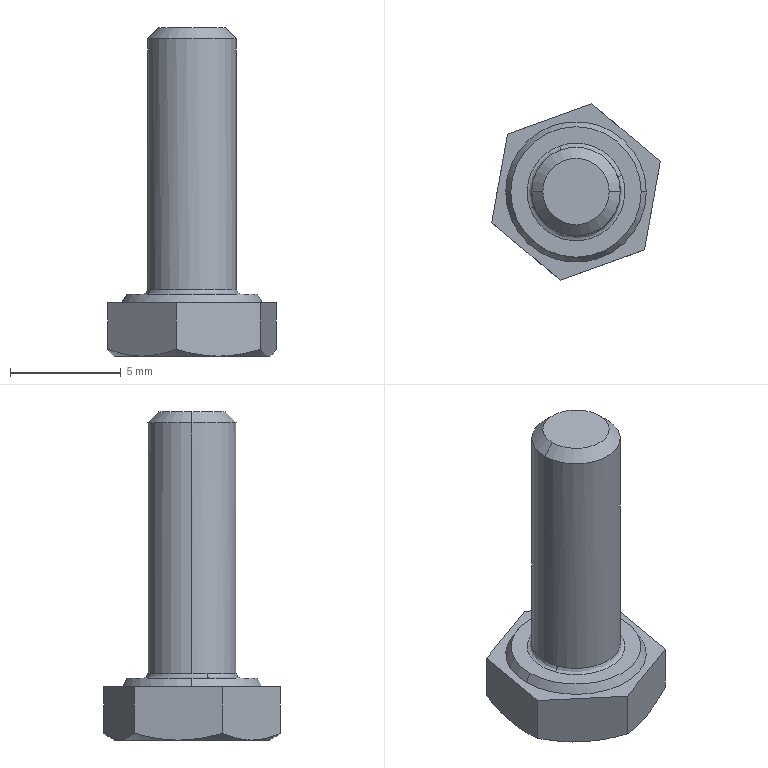Part | NX | features BREP 1 | 1 solid | 39 faces | box 7.602 x 7.957 x 14.8 mm | volume 249.931 mm3 | plane 23 | cone 11 | spline 3 | cylinder 2 | commonest cylinder face diameters 4 x2
STEP:
#1=CARTESIAN_POINT('',(-262.311,-178.403,2116.));
#2=VERTEX_POINT('',#1);
#3=CARTESIAN_POINT('',(-258.311,-178.403,2116.));
#4=VERTEX_POINT('',#3);
#5=CARTESIAN_POINT('',(-260.311,-178.403,2116.));
#6=DIRECTION('',(0.,0.,-1.));
#7=DIRECTION('',(-1.,0.,0.));
#8=AXIS2_PLACEMENT_3D('',#5,#6,#7);
#9=CIRCLE('',#8,2.);
#10=EDGE_CURVE('',#2,#4,#9,.T.);
#11=ORIENTED_EDGE('',*,*,#10,.T.);
#12=CARTESIAN_POINT('',(-258.311,-178.403,2104.7));
#13=VERTEX_POINT('',#12);
#14=CARTESIAN_POINT('',(-258.311,-178.403,2101.7));
#15=DIRECTION('',(0.,0.,-1.));
#16=VECTOR('',#15,1000.);
#17=LINE('',#14,#16);
#18=EDGE_CURVE('',#13,#4,#17,.F.);
#19=ORIENTED_EDGE('',*,*,#18,.F.);
#20=CARTESIAN_POINT('',(-258.429,-177.724,2104.7));
#21=VERTEX_POINT('',#20);
#22=CARTESIAN_POINT('',(-260.311,-178.403,2104.7));
#23=DIRECTION('',(0.,0.,1.));
#24=DIRECTION('',(-1.,0.,0.));
#25=AXIS2_PLACEMENT_3D('',#22,#23,#24);
#26=CIRCLE('',#25,2.);
#27=EDGE_CURVE('',#13,#21,#26,.T.);
#28=ORIENTED_EDGE('',*,*,#27,.T.);
#29=CARTESIAN_POINT('',(-260.99,-176.522,2104.7));
#30=VERTEX_POINT('',#29);
#31=CARTESIAN_POINT('',(-260.311,-178.403,2104.7));
#32=DIRECTION('',(0.,0.,1.));
#33=DIRECTION('',(-1.,0.,0.));
#34=AXIS2_PLACEMENT_3D('',#31,#32,#33);
#35=CIRCLE('',#34,2.);
#36=EDGE_CURVE('',#21,#30,#35,.T.);
#37=ORIENTED_EDGE('',*,*,#36,.T.);
#38=CARTESIAN_POINT('',(-262.311,-178.403,2104.7));
#39=VERTEX_POINT('',#38);
#40=CARTESIAN_POINT('',(-260.311,-178.403,2104.7));
#41=DIRECTION('',(0.,0.,1.));
#42=DIRECTION('',(-1.,0.,0.));
#43=AXIS2_PLACEMENT_3D('',#40,#41,#42);
#44=CIRCLE('',#43,2.);
#45=EDGE_CURVE('',#30,#39,#44,.T.);
#46=ORIENTED_EDGE('',*,*,#45,.T.);
#47=CARTESIAN_POINT('',(-262.311,-178.403,2101.7));
#48=DIRECTION('',(0.,0.,-1.));
#49=VECTOR('',#48,1000.);
#50=LINE('',#47,#49);
#51=EDGE_CURVE('',#39,#2,#50,.F.);
#52=ORIENTED_EDGE('',*,*,#51,.T.);
#53=EDGE_LOOP('',(#11,#19,#28,#37,#46,#52));
#54=FACE_BOUND('',#53,.T.);
#55=CARTESIAN_POINT('',(-260.311,-178.403,2101.7));
#56=DIRECTION('',(0.,0.,-1.));
#57=DIRECTION('',(1.,0.,0.));
#58=AXIS2_PLACEMENT_3D('',#55,#56,#57);
#59=CYLINDRICAL_SURFACE('',#58,2.);
#60=ADVANCED_FACE('',(#54),#59,.T.);
#61=CARTESIAN_POINT('',(-261.811,-178.403,2116.5));
#62=VERTEX_POINT('',#61);
#63=CARTESIAN_POINT('',(-258.811,-178.403,2116.5));
#64=VERTEX_POINT('',#63);
#65=CARTESIAN_POINT('',(-260.311,-178.403,2116.5));
#66=DIRECTION('',(0.,0.,-1.));
#67=DIRECTION('',(-1.,0.,0.));
#68=AXIS2_PLACEMENT_3D('',#65,#66,#67);
#69=CIRCLE('',#68,1.5);
#70=EDGE_CURVE('',#62,#64,#69,.T.);
#71=ORIENTED_EDGE('',*,*,#70,.T.);
#72=CARTESIAN_POINT('',(-258.311,-178.403,2116.));
#73=DIRECTION('',(0.7071,0.,-0.7071));
#74=VECTOR('',#73,1000.);
#75=LINE('',#72,#74);
#76=EDGE_CURVE('',#4,#64,#75,.F.);
#77=ORIENTED_EDGE('',*,*,#76,.F.);
#78=ORIENTED_EDGE('',*,*,#10,.F.);
#79=CARTESIAN_POINT('',(-262.311,-178.403,2116.));
#80=DIRECTION('',(-0.7071,0.,-0.7071));
#81=VECTOR('',#80,1000.);
#82=LINE('',#79,#81);
#83=EDGE_CURVE('',#2,#62,#82,.F.);
#84=ORIENTED_EDGE('',*,*,#83,.T.);
#85=EDGE_LOOP('',(#71,#77,#78,#84));
#86=FACE_BOUND('',#85,.T.);
#87=CARTESIAN_POINT('',(-260.311,-178.403,2116.));
#88=DIRECTION('',(0.,0.,-1.));
#89=DIRECTION('',(1.,0.,0.));
#90=AXIS2_PLACEMENT_3D('',#87,#88,#89);
#91=CONICAL_SURFACE('',#90,2.,0.7854);
#92=ADVANCED_FACE('',(#86),#91,.T.);
#93=CARTESIAN_POINT('',(-257.371,-178.403,2104.5));
#94=VERTEX_POINT('',#93);
#95=CARTESIAN_POINT('',(-263.251,-178.403,2104.5));
#96=VERTEX_POINT('',#95);
#97=CARTESIAN_POINT('',(-260.311,-178.403,2104.5));
#98=DIRECTION('',(0.,0.,1.));
#99=DIRECTION('',(-1.,0.,0.));
#100=AXIS2_PLACEMENT_3D('',#97,#98,#99);
#101=CIRCLE('',#100,2.94);
#102=EDGE_CURVE('',#94,#96,#101,.T.);
#103=ORIENTED_EDGE('',*,*,#102,.F.);
#104=CARTESIAN_POINT('',(-257.14,-178.403,2104.1));
#105=VERTEX_POINT('',#104);
#106=CARTESIAN_POINT('',(-257.14,-178.403,2104.1));
#107=DIRECTION('',(0.5,0.,-0.866));
#108=VECTOR('',#107,1000.);
#109=LINE('',#106,#108);
#110=EDGE_CURVE('',#105,#94,#109,.F.);
#111=ORIENTED_EDGE('',*,*,#110,.F.);
#112=CARTESIAN_POINT('',(-263.481,-178.403,2104.1));
#113=VERTEX_POINT('',#112);
#114=CARTESIAN_POINT('',(-260.311,-178.403,2104.1));
#115=DIRECTION('',(0.,0.,1.));
#116=DIRECTION('',(-1.,0.,0.));
#117=AXIS2_PLACEMENT_3D('',#114,#115,#116);
#118=CIRCLE('',#117,3.171);
#119=EDGE_CURVE('',#105,#113,#118,.T.);
#120=ORIENTED_EDGE('',*,*,#119,.T.);
#121=CARTESIAN_POINT('',(-263.481,-178.403,2104.1));
#122=DIRECTION('',(-0.5,0.,-0.866));
#123=VECTOR('',#122,1000.);
#124=LINE('',#121,#123);
#125=EDGE_CURVE('',#113,#96,#124,.F.);
#126=ORIENTED_EDGE('',*,*,#125,.T.);
#127=EDGE_LOOP('',(#103,#111,#120,#126));
#128=FACE_BOUND('',#127,.T.);
#129=CARTESIAN_POINT('',(-260.311,-178.403,2104.1));
#130=DIRECTION('',(0.,0.,-1.));
#131=DIRECTION('',(1.,0.,0.));
#132=AXIS2_PLACEMENT_3D('',#129,#130,#131);
#133=CONICAL_SURFACE('',#132,3.171,0.5236);
#134=ADVANCED_FACE('',(#128),#133,.T.);
#135=CARTESIAN_POINT('',(-256.865,-179.019,2101.7));
#136=VERTEX_POINT('',#135);
#137=CARTESIAN_POINT('',(-256.811,-178.403,2101.7));
#138=VERTEX_POINT('',#137);
#139=CARTESIAN_POINT('',(-260.311,-178.403,2101.7));
#140=DIRECTION('',(0.,0.,1.));
#141=DIRECTION('',(1.,0.,0.));
#142=AXIS2_PLACEMENT_3D('',#139,#140,#141);
#143=CIRCLE('',#142,3.5);
#144=EDGE_CURVE('',#136,#138,#143,.T.);
#145=ORIENTED_EDGE('',*,*,#144,.T.);
#146=CARTESIAN_POINT('',(-256.755,-178.403,2101.732));
#147=VERTEX_POINT('',#146);
#148=CARTESIAN_POINT('',(-256.266,-178.403,2102.014));
#149=DIRECTION('',(0.866,0.,0.5));
#150=VECTOR('',#149,1000.);
#151=LINE('',#148,#150);
#152=EDGE_CURVE('',#138,#147,#151,.T.);
#153=ORIENTED_EDGE('',*,*,#152,.T.);
#154=CARTESIAN_POINT('',(-256.755,-178.403,2101.732));
#155=CARTESIAN_POINT('',(-256.792,-178.608,2101.711));
#156=CARTESIAN_POINT('',(-256.828,-178.813,2101.7));
#157=CARTESIAN_POINT('',(-256.865,-179.019,2101.7));
#158=B_SPLINE_CURVE_WITH_KNOTS('',3,(#154,#155,#156,#157),.UNSPECIFIED.,.F.,.F.,(4,4),(0.,0.0006269),.UNSPECIFIED.);
#159=EDGE_CURVE('',#147,#136,#158,.T.);
#160=ORIENTED_EDGE('',*,*,#159,.T.);
#161=EDGE_LOOP('',(#145,#153,#160));
#162=FACE_BOUND('',#161,.T.);
#163=CARTESIAN_POINT('',(-260.311,-178.403,2102.014));
#164=DIRECTION('',(0.,0.,1.));
#165=DIRECTION('',(-1.,0.,0.));
#166=AXIS2_PLACEMENT_3D('',#163,#164,#165);
#167=CONICAL_SURFACE('',#166,4.045,1.047);
#168=ADVANCED_FACE('',(#162),#167,.T.);
#169=ORIENTED_EDGE('',*,*,#18,.T.);
#170=CARTESIAN_POINT('',(-260.311,-178.403,2116.));
#171=DIRECTION('',(0.,0.,-1.));
#172=DIRECTION('',(-1.,0.,0.));
#173=AXIS2_PLACEMENT_3D('',#170,#171,#172);
#174=CIRCLE('',#173,2.);
#175=EDGE_CURVE('',#4,#2,#174,.T.);
#176=ORIENTED_EDGE('',*,*,#175,.T.);
#177=ORIENTED_EDGE('',*,*,#51,.F.);
#178=CARTESIAN_POINT('',(-262.192,-179.082,2104.7));
#179=VERTEX_POINT('',#178);
#180=CARTESIAN_POINT('',(-260.311,-178.403,2104.7));
#181=DIRECTION('',(0.,0.,1.));
#182=DIRECTION('',(-1.,0.,0.));
#183=AXIS2_PLACEMENT_3D('',#180,#181,#182);
#184=CIRCLE('',#183,2.);
#185=EDGE_CURVE('',#39,#179,#184,.T.);
#186=ORIENTED_EDGE('',*,*,#185,.T.);
#187=CARTESIAN_POINT('',(-260.311,-178.403,2104.7));
#188=DIRECTION('',(0.,0.,1.));
#189=DIRECTION('',(-1.,0.,0.));
#190=AXIS2_PLACEMENT_3D('',#187,#188,#189);
#191=CIRCLE('',#190,2.);
#192=EDGE_CURVE('',#179,#13,#191,.T.);
#193=ORIENTED_EDGE('',*,*,#192,.T.);
#194=EDGE_LOOP('',(#169,#176,#177,#186,#193));
#195=FACE_BOUND('',#194,.T.);
#196=CARTESIAN_POINT('',(-260.311,-178.403,2101.7));
#197=DIRECTION('',(0.,0.,-1.));
#198=DIRECTION('',(1.,0.,0.));
#199=AXIS2_PLACEMENT_3D('',#196,#197,#198);
#200=CYLINDRICAL_SURFACE('',#199,2.);
#201=ADVANCED_FACE('',(#195),#200,.T.);
#202=CARTESIAN_POINT('',(-262.51,-178.336,2104.5));
#203=VERTEX_POINT('',#202);
#204=CARTESIAN_POINT('',(-262.302,-177.469,2104.5));
#205=VERTEX_POINT('',#204);
#206=CARTESIAN_POINT('',(-262.51,-178.336,2104.5));
#207=CARTESIAN_POINT('',(-262.501,-178.033,2104.5));
#208=CARTESIAN_POINT('',(-262.432,-177.744,2104.5));
#209=CARTESIAN_POINT('',(-262.302,-177.469,2104.5));
#210=B_SPLINE_CURVE_WITH_KNOTS('',3,(#206,#207,#208,#209),.UNSPECIFIED.,.F.,.F.,(4,4),(0.,1.),.PIECEWISE_BEZIER_KNOTS.);
#211=EDGE_CURVE('',#203,#205,#210,.T.);
#212=ORIENTED_EDGE('',*,*,#211,.F.);
#213=CARTESIAN_POINT('',(-262.38,-179.149,2104.5));
#214=VERTEX_POINT('',#213);
#215=CARTESIAN_POINT('',(-262.38,-179.149,2104.5));
#216=CARTESIAN_POINT('',(-262.475,-178.886,2104.5));
#217=CARTESIAN_POINT('',(-262.518,-178.615,2104.5));
#218=CARTESIAN_POINT('',(-262.51,-178.336,2104.5));
#219=B_SPLINE_CURVE_WITH_KNOTS('',3,(#215,#216,#217,#218),.UNSPECIFIED.,.F.,.F.,(4,4),(0.,1.),.PIECEWISE_BEZIER_KNOTS.);
#220=EDGE_CURVE('',#214,#203,#219,.T.);
#221=ORIENTED_EDGE('',*,*,#220,.F.);
#222=CARTESIAN_POINT('',(-262.38,-179.15,2104.5));
#223=VERTEX_POINT('',#222);
#224=CARTESIAN_POINT('',(-262.38,-179.15,2104.5));
#225=DIRECTION('',(-0.3394,0.9407,-0.000009634));
#226=VECTOR('',#225,1000.);
#227=LINE('',#224,#226);
#228=EDGE_CURVE('',#223,#214,#227,.T.);
#229=ORIENTED_EDGE('',*,*,#228,.F.);
#230=CARTESIAN_POINT('',(-262.192,-179.082,2104.7));
#231=CARTESIAN_POINT('',(-262.192,-179.082,2104.583));
#232=CARTESIAN_POINT('',(-262.269,-179.11,2104.5));
#233=CARTESIAN_POINT('',(-262.38,-179.15,2104.5));
#234=(BOUNDED_CURVE()B_SPLINE_CURVE(3,(#230,#231,#232,#233),.UNSPECIFIED.,.F.,.F.)B_SPLINE_CURVE_WITH_KNOTS((4,4),(0.,1.),.PIECEWISE_BEZIER_KNOTS.)CURVE()GEOMETRIC_REPRESENTATION_ITEM()RATIONAL_B_SPLINE_CURVE((1.,0.8034,0.8016,0.9945))REPRESENTATION_ITEM(''));
#235=EDGE_CURVE('',#179,#223,#234,.T.);
#236=ORIENTED_EDGE('',*,*,#235,.F.);
#237=ORIENTED_EDGE('',*,*,#185,.F.);
#238=ORIENTED_EDGE('',*,*,#45,.F.);
#239=CARTESIAN_POINT('',(-261.057,-176.334,2104.5));
#240=VERTEX_POINT('',#239);
#241=CARTESIAN_POINT('',(-260.99,-176.522,2104.7));
#242=CARTESIAN_POINT('',(-260.99,-176.522,2104.606));
#243=CARTESIAN_POINT('',(-261.026,-176.422,2104.5));
#244=CARTESIAN_POINT('',(-261.057,-176.334,2104.5));
#245=B_SPLINE_CURVE_WITH_KNOTS('',3,(#241,#242,#243,#244),.UNSPECIFIED.,.F.,.F.,(4,4),(0.,1.),.UNSPECIFIED.);
#246=EDGE_CURVE('',#240,#30,#245,.F.);
#247=ORIENTED_EDGE('',*,*,#246,.F.);
#248=CARTESIAN_POINT('',(-261.768,-176.755,2104.5));
#249=VERTEX_POINT('',#248);
#250=CARTESIAN_POINT('',(-261.768,-176.755,2104.5));
#251=CARTESIAN_POINT('',(-261.558,-176.569,2104.5));
#252=CARTESIAN_POINT('',(-261.321,-176.429,2104.5));
#253=CARTESIAN_POINT('',(-261.057,-176.334,2104.5));
#254=B_SPLINE_CURVE_WITH_KNOTS('',3,(#250,#251,#252,#253),.UNSPECIFIED.,.F.,.F.,(4,4),(0.,1.),.PIECEWISE_BEZIER_KNOTS.);
#255=EDGE_CURVE('',#249,#240,#254,.T.);
#256=ORIENTED_EDGE('',*,*,#255,.F.);
#257=CARTESIAN_POINT('',(-262.302,-177.469,2104.5));
#258=CARTESIAN_POINT('',(-262.174,-177.194,2104.5));
#259=CARTESIAN_POINT('',(-261.995,-176.956,2104.5));
#260=CARTESIAN_POINT('',(-261.768,-176.755,2104.5));
#261=B_SPLINE_CURVE_WITH_KNOTS('',3,(#257,#258,#259,#260),.UNSPECIFIED.,.F.,.F.,(4,4),(0.,1.),.PIECEWISE_BEZIER_KNOTS.);
#262=EDGE_CURVE('',#205,#249,#261,.T.);
#263=ORIENTED_EDGE('',*,*,#262,.F.);
#264=EDGE_LOOP('',(#212,#221,#229,#236,#237,#238,#247,#256,#263));
#265=FACE_BOUND('',#264,.T.);
#266=CARTESIAN_POINT('',(-261.041,-176.325,2104.5));
#267=CARTESIAN_POINT('',(-261.047,-176.327,2104.5));
#268=CARTESIAN_POINT('',(-261.053,-176.33,2104.5));
#269=CARTESIAN_POINT('',(-261.059,-176.332,2104.5));
#270=CARTESIAN_POINT('',(-262.272,-176.77,2104.5));
#271=CARTESIAN_POINT('',(-262.82,-177.938,2104.5));
#272=CARTESIAN_POINT('',(-262.382,-179.151,2104.5));
#273=CARTESIAN_POINT('',(-261.001,-176.437,2104.499));
#274=CARTESIAN_POINT('',(-261.007,-176.439,2104.499));
#275=CARTESIAN_POINT('',(-261.013,-176.441,2104.499));
#276=CARTESIAN_POINT('',(-261.018,-176.443,2104.499));
#277=CARTESIAN_POINT('',(-262.167,-176.858,2104.499));
#278=CARTESIAN_POINT('',(-262.685,-177.963,2104.499));
#279=CARTESIAN_POINT('',(-262.271,-179.111,2104.499));
#280=CARTESIAN_POINT('',(-260.974,-176.516,2104.582));
#281=CARTESIAN_POINT('',(-260.979,-176.518,2104.582));
#282=CARTESIAN_POINT('',(-260.984,-176.52,2104.582));
#283=CARTESIAN_POINT('',(-260.99,-176.522,2104.582));
#284=CARTESIAN_POINT('',(-262.092,-176.92,2104.582));
#285=CARTESIAN_POINT('',(-262.59,-177.98,2104.582));
#286=CARTESIAN_POINT('',(-262.192,-179.082,2104.582));
#287=CARTESIAN_POINT('',(-260.974,-176.516,2104.7));
#288=CARTESIAN_POINT('',(-260.979,-176.518,2104.7));
#289=CARTESIAN_POINT('',(-260.984,-176.52,2104.7));
#290=CARTESIAN_POINT('',(-260.99,-176.522,2104.7));
#291=CARTESIAN_POINT('',(-262.092,-176.92,2104.7));
#292=CARTESIAN_POINT('',(-262.59,-177.98,2104.7));
#293=CARTESIAN_POINT('',(-262.192,-179.082,2104.7));
#294=(BOUNDED_SURFACE()B_SPLINE_SURFACE(3,3,((#266,#267,#268,#269,#270,#271,#272),(#273,#274,#275,#276,#277,#278,#279),(#280,#281,#282,#283,#284,#285,#286),(#287,#288,#289,#290,#291,#292,#293)),.UNSPECIFIED.,.F.,.F.,.F.)B_SPLINE_SURFACE_WITH_KNOTS((4,4),(4,3,4),(0.,1.),(0.003818,0.009901,1.),.PIECEWISE_BEZIER_KNOTS.)GEOMETRIC_REPRESENTATION_ITEM()RATIONAL_B_SPLINE_SURFACE(((1.,1.,1.,1.,0.8047,0.8047,1.),(0.8022,0.8022,0.8022,0.8022,0.6456,0.6456,0.8022),(0.8022,0.8022,0.8022,0.8022,0.6456,0.6456,0.8022),(1.,1.,1.,1.,0.8047,0.8047,1.)))REPRESENTATION_ITEM('')SURFACE());
#295=ADVANCED_FACE('',(#265),#294,.F.);
#296=CARTESIAN_POINT('',(-258.663,-176.945,2104.5));
#297=VERTEX_POINT('',#296);
#298=CARTESIAN_POINT('',(-258.241,-177.656,2104.5));
#299=VERTEX_POINT('',#298);
#300=CARTESIAN_POINT('',(-258.663,-176.945,2104.5));
#301=CARTESIAN_POINT('',(-258.476,-177.156,2104.5));
#302=CARTESIAN_POINT('',(-258.336,-177.393,2104.5));
#303=CARTESIAN_POINT('',(-258.241,-177.656,2104.5));
#304=B_SPLINE_CURVE_WITH_KNOTS('',3,(#300,#301,#302,#303),.UNSPECIFIED.,.F.,.F.,(4,4),(0.,1.),.PIECEWISE_BEZIER_KNOTS.);
#305=EDGE_CURVE('',#297,#299,#304,.T.);
#306=ORIENTED_EDGE('',*,*,#305,.F.);
#307=CARTESIAN_POINT('',(-259.376,-176.411,2104.5));
#308=VERTEX_POINT('',#307);
#309=CARTESIAN_POINT('',(-259.376,-176.411,2104.5));
#310=CARTESIAN_POINT('',(-259.102,-176.54,2104.5));
#311=CARTESIAN_POINT('',(-258.864,-176.718,2104.5));
#312=CARTESIAN_POINT('',(-258.663,-176.945,2104.5));
#313=B_SPLINE_CURVE_WITH_KNOTS('',3,(#309,#310,#311,#312),.UNSPECIFIED.,.F.,.F.,(4,4),(0.,1.),.PIECEWISE_BEZIER_KNOTS.);
#314=EDGE_CURVE('',#308,#297,#313,.T.);
#315=ORIENTED_EDGE('',*,*,#314,.F.);
#316=CARTESIAN_POINT('',(-260.243,-176.204,2104.5));
#317=VERTEX_POINT('',#316);
#318=CARTESIAN_POINT('',(-260.243,-176.204,2104.5));
#319=CARTESIAN_POINT('',(-259.94,-176.213,2104.5));
#320=CARTESIAN_POINT('',(-259.651,-176.282,2104.5));
#321=CARTESIAN_POINT('',(-259.376,-176.411,2104.5));
#322=B_SPLINE_CURVE_WITH_KNOTS('',3,(#318,#319,#320,#321),.UNSPECIFIED.,.F.,.F.,(4,4),(0.,1.),.PIECEWISE_BEZIER_KNOTS.);
#323=EDGE_CURVE('',#317,#308,#322,.T.);
#324=ORIENTED_EDGE('',*,*,#323,.F.);
#325=CARTESIAN_POINT('',(-261.057,-176.334,2104.5));
#326=CARTESIAN_POINT('',(-260.795,-176.239,2104.5));
#327=CARTESIAN_POINT('',(-260.523,-176.195,2104.5));
#328=CARTESIAN_POINT('',(-260.243,-176.204,2104.5));
#329=B_SPLINE_CURVE_WITH_KNOTS('',3,(#325,#326,#327,#328),.UNSPECIFIED.,.F.,.F.,(4,4),(0.,1.),.PIECEWISE_BEZIER_KNOTS.);
#330=EDGE_CURVE('',#240,#317,#329,.T.);
#331=ORIENTED_EDGE('',*,*,#330,.F.);
#332=ORIENTED_EDGE('',*,*,#246,.T.);
#333=ORIENTED_EDGE('',*,*,#36,.F.);
#334=CARTESIAN_POINT('',(-258.241,-177.656,2104.5));
#335=CARTESIAN_POINT('',(-258.352,-177.695,2104.5));
#336=CARTESIAN_POINT('',(-258.429,-177.724,2104.583));
#337=CARTESIAN_POINT('',(-258.429,-177.724,2104.7));
#338=(BOUNDED_CURVE()B_SPLINE_CURVE(3,(#334,#335,#336,#337),.UNSPECIFIED.,.F.,.F.)B_SPLINE_CURVE_WITH_KNOTS((4,4),(0.,1.),.PIECEWISE_BEZIER_KNOTS.)CURVE()GEOMETRIC_REPRESENTATION_ITEM()RATIONAL_B_SPLINE_CURVE((0.9949,0.8016,0.8032,1.))REPRESENTATION_ITEM(''));
#339=EDGE_CURVE('',#299,#21,#338,.T.);
#340=ORIENTED_EDGE('',*,*,#339,.F.);
#341=EDGE_LOOP('',(#306,#315,#324,#331,#332,#333,#340));
#342=FACE_BOUND('',#341,.T.);
#343=CARTESIAN_POINT('',(-258.239,-177.655,2104.5));
#344=CARTESIAN_POINT('',(-258.678,-176.442,2104.5));
#345=CARTESIAN_POINT('',(-259.845,-175.894,2104.5));
#346=CARTESIAN_POINT('',(-261.059,-176.332,2104.5));
#347=CARTESIAN_POINT('',(-258.35,-177.695,2104.499));
#348=CARTESIAN_POINT('',(-258.765,-176.547,2104.499));
#349=CARTESIAN_POINT('',(-259.87,-176.028,2104.499));
#350=CARTESIAN_POINT('',(-261.018,-176.443,2104.499));
#351=CARTESIAN_POINT('',(-258.429,-177.724,2104.582));
#352=CARTESIAN_POINT('',(-258.827,-176.622,2104.582));
#353=CARTESIAN_POINT('',(-259.888,-176.124,2104.582));
#354=CARTESIAN_POINT('',(-260.99,-176.522,2104.582));
#355=CARTESIAN_POINT('',(-258.429,-177.724,2104.7));
#356=CARTESIAN_POINT('',(-258.827,-176.622,2104.7));
#357=CARTESIAN_POINT('',(-259.888,-176.124,2104.7));
#358=CARTESIAN_POINT('',(-260.99,-176.522,2104.7));
#359=(BOUNDED_SURFACE()B_SPLINE_SURFACE(3,3,((#343,#344,#345,#346),(#347,#348,#349,#350),(#351,#352,#353,#354),(#355,#356,#357,#358)),.UNSPECIFIED.,.F.,.F.,.F.)B_SPLINE_SURFACE_WITH_KNOTS((4,4),(4,4),(0.,1.),(0.,1.),.PIECEWISE_BEZIER_KNOTS.)GEOMETRIC_REPRESENTATION_ITEM()RATIONAL_B_SPLINE_SURFACE(((1.,0.8047,0.8047,1.),(0.8022,0.6456,0.6456,0.8022),(0.8022,0.6456,0.6456,0.8022),(1.,0.8047,0.8047,1.)))REPRESENTATION_ITEM('')SURFACE());
#360=ADVANCED_FACE('',(#342),#359,.F.);
#361=ORIENTED_EDGE('',*,*,#76,.T.);
#362=CARTESIAN_POINT('',(-260.311,-178.403,2116.5));
#363=DIRECTION('',(0.,0.,-1.));
#364=DIRECTION('',(-1.,0.,0.));
#365=AXIS2_PLACEMENT_3D('',#362,#363,#364);
#366=CIRCLE('',#365,1.5);
#367=EDGE_CURVE('',#64,#62,#366,.T.);
#368=ORIENTED_EDGE('',*,*,#367,.T.);
#369=ORIENTED_EDGE('',*,*,#83,.F.);
#370=ORIENTED_EDGE('',*,*,#175,.F.);
#371=EDGE_LOOP('',(#361,#368,#369,#370));
#372=FACE_BOUND('',#371,.T.);
#373=CARTESIAN_POINT('',(-260.311,-178.403,2116.));
#374=DIRECTION('',(0.,0.,-1.));
#375=DIRECTION('',(1.,0.,0.));
#376=AXIS2_PLACEMENT_3D('',#373,#374,#375);
#377=CONICAL_SURFACE('',#376,2.,0.7854);
#378=ADVANCED_FACE('',(#372),#377,.T.);
#379=CARTESIAN_POINT('',(-261.245,-180.395,2104.5));
#380=VERTEX_POINT('',#379);
#381=CARTESIAN_POINT('',(-261.958,-179.861,2104.5));
#382=VERTEX_POINT('',#381);
#383=CARTESIAN_POINT('',(-261.245,-180.395,2104.5));
#384=CARTESIAN_POINT('',(-261.519,-180.266,2104.5));
#385=CARTESIAN_POINT('',(-261.757,-180.088,2104.5));
#386=CARTESIAN_POINT('',(-261.958,-179.861,2104.5));
#387=B_SPLINE_CURVE_WITH_KNOTS('',3,(#383,#384,#385,#386),.UNSPECIFIED.,.F.,.F.,(4,4),(0.,1.),.PIECEWISE_BEZIER_KNOTS.);
#388=EDGE_CURVE('',#380,#382,#387,.T.);
#389=ORIENTED_EDGE('',*,*,#388,.F.);
#390=CARTESIAN_POINT('',(-260.378,-180.602,2104.5));
#391=VERTEX_POINT('',#390);
#392=CARTESIAN_POINT('',(-260.378,-180.602,2104.5));
#393=CARTESIAN_POINT('',(-260.681,-180.593,2104.5));
#394=CARTESIAN_POINT('',(-260.97,-180.524,2104.5));
#395=CARTESIAN_POINT('',(-261.245,-180.395,2104.5));
#396=B_SPLINE_CURVE_WITH_KNOTS('',3,(#392,#393,#394,#395),.UNSPECIFIED.,.F.,.F.,(4,4),(0.,1.),.PIECEWISE_BEZIER_KNOTS.);
#397=EDGE_CURVE('',#391,#380,#396,.T.);
#398=ORIENTED_EDGE('',*,*,#397,.F.);
#399=CARTESIAN_POINT('',(-259.564,-180.473,2104.5));
#400=VERTEX_POINT('',#399);
#401=CARTESIAN_POINT('',(-259.564,-180.473,2104.5));
#402=CARTESIAN_POINT('',(-259.827,-180.567,2104.5));
#403=CARTESIAN_POINT('',(-260.098,-180.611,2104.5));
#404=CARTESIAN_POINT('',(-260.378,-180.602,2104.5));
#405=B_SPLINE_CURVE_WITH_KNOTS('',3,(#401,#402,#403,#404),.UNSPECIFIED.,.F.,.F.,(4,4),(0.,1.),.PIECEWISE_BEZIER_KNOTS.);
#406=EDGE_CURVE('',#400,#391,#405,.T.);
#407=ORIENTED_EDGE('',*,*,#406,.F.);
#408=CARTESIAN_POINT('',(-258.853,-180.051,2104.5));
#409=VERTEX_POINT('',#408);
#410=CARTESIAN_POINT('',(-258.853,-180.051,2104.5));
#411=CARTESIAN_POINT('',(-259.064,-180.237,2104.5));
#412=CARTESIAN_POINT('',(-259.3,-180.378,2104.5));
#413=CARTESIAN_POINT('',(-259.564,-180.473,2104.5));
#414=B_SPLINE_CURVE_WITH_KNOTS('',3,(#410,#411,#412,#413),.UNSPECIFIED.,.F.,.F.,(4,4),(0.,1.),.PIECEWISE_BEZIER_KNOTS.);
#415=EDGE_CURVE('',#409,#400,#414,.T.);
#416=ORIENTED_EDGE('',*,*,#415,.F.);
#417=CARTESIAN_POINT('',(-258.319,-179.337,2104.5));
#418=VERTEX_POINT('',#417);
#419=CARTESIAN_POINT('',(-258.319,-179.337,2104.5));
#420=CARTESIAN_POINT('',(-258.447,-179.612,2104.5));
#421=CARTESIAN_POINT('',(-258.626,-179.85,2104.5));
#422=CARTESIAN_POINT('',(-258.853,-180.051,2104.5));
#423=B_SPLINE_CURVE_WITH_KNOTS('',3,(#419,#420,#421,#422),.UNSPECIFIED.,.F.,.F.,(4,4),(0.,1.),.PIECEWISE_BEZIER_KNOTS.);
#424=EDGE_CURVE('',#418,#409,#423,.T.);
#425=ORIENTED_EDGE('',*,*,#424,.F.);
#426=CARTESIAN_POINT('',(-258.111,-178.47,2104.5));
#427=VERTEX_POINT('',#426);
#428=CARTESIAN_POINT('',(-258.111,-178.47,2104.5));
#429=CARTESIAN_POINT('',(-258.12,-178.773,2104.5));
#430=CARTESIAN_POINT('',(-258.189,-179.062,2104.5));
#431=CARTESIAN_POINT('',(-258.319,-179.337,2104.5));
#432=B_SPLINE_CURVE_WITH_KNOTS('',3,(#428,#429,#430,#431),.UNSPECIFIED.,.F.,.F.,(4,4),(0.,1.),.PIECEWISE_BEZIER_KNOTS.);
#433=EDGE_CURVE('',#427,#418,#432,.T.);
#434=ORIENTED_EDGE('',*,*,#433,.F.);
#435=CARTESIAN_POINT('',(-258.241,-177.657,2104.5));
#436=VERTEX_POINT('',#435);
#437=CARTESIAN_POINT('',(-258.241,-177.657,2104.5));
#438=CARTESIAN_POINT('',(-258.146,-177.919,2104.5));
#439=CARTESIAN_POINT('',(-258.103,-178.19,2104.5));
#440=CARTESIAN_POINT('',(-258.111,-178.47,2104.5));
#441=B_SPLINE_CURVE_WITH_KNOTS('',3,(#437,#438,#439,#440),.UNSPECIFIED.,.F.,.F.,(4,4),(0.,1.),.PIECEWISE_BEZIER_KNOTS.);
#442=EDGE_CURVE('',#436,#427,#441,.T.);
#443=ORIENTED_EDGE('',*,*,#442,.F.);
#444=CARTESIAN_POINT('',(-258.241,-177.656,2104.5));
#445=CARTESIAN_POINT('',(-258.241,-177.656,2104.5));
#446=CARTESIAN_POINT('',(-258.241,-177.656,2104.5));
#447=CARTESIAN_POINT('',(-258.241,-177.657,2104.5));
#448=B_SPLINE_CURVE_WITH_KNOTS('',3,(#444,#445,#446,#447),.UNSPECIFIED.,.F.,.F.,(4,4),(0.,1.),.PIECEWISE_BEZIER_KNOTS.);
#449=EDGE_CURVE('',#299,#436,#448,.T.);
#450=ORIENTED_EDGE('',*,*,#449,.F.);
#451=ORIENTED_EDGE('',*,*,#339,.T.);
#452=ORIENTED_EDGE('',*,*,#27,.F.);
#453=ORIENTED_EDGE('',*,*,#192,.F.);
#454=ORIENTED_EDGE('',*,*,#235,.T.);
#455=CARTESIAN_POINT('',(-261.958,-179.861,2104.5));
#456=CARTESIAN_POINT('',(-262.145,-179.65,2104.5));
#457=CARTESIAN_POINT('',(-262.285,-179.413,2104.5));
#458=CARTESIAN_POINT('',(-262.38,-179.15,2104.5));
#459=B_SPLINE_CURVE_WITH_KNOTS('',3,(#455,#456,#457,#458),.UNSPECIFIED.,.F.,.F.,(4,4),(0.,1.),.PIECEWISE_BEZIER_KNOTS.);
#460=EDGE_CURVE('',#382,#223,#459,.T.);
#461=ORIENTED_EDGE('',*,*,#460,.F.);
#462=EDGE_LOOP('',(#389,#398,#407,#416,#425,#434,#443,#450,#451,#452,#453,#454,#461));
#463=FACE_BOUND('',#462,.T.);
#464=CARTESIAN_POINT('',(-262.382,-179.151,2104.5));
#465=CARTESIAN_POINT('',(-260.886,-183.294,2104.5));
#466=CARTESIAN_POINT('',(-256.743,-181.798,2104.5));
#467=CARTESIAN_POINT('',(-258.239,-177.655,2104.5));
#468=CARTESIAN_POINT('',(-262.271,-179.111,2104.499));
#469=CARTESIAN_POINT('',(-260.855,-183.031,2104.499));
#470=CARTESIAN_POINT('',(-256.934,-181.615,2104.499));
#471=CARTESIAN_POINT('',(-258.35,-177.695,2104.499));
#472=CARTESIAN_POINT('',(-262.192,-179.082,2104.582));
#473=CARTESIAN_POINT('',(-260.833,-182.845,2104.582));
#474=CARTESIAN_POINT('',(-257.071,-181.486,2104.582));
#475=CARTESIAN_POINT('',(-258.429,-177.724,2104.582));
#476=CARTESIAN_POINT('',(-262.192,-179.082,2104.7));
#477=CARTESIAN_POINT('',(-260.833,-182.845,2104.7));
#478=CARTESIAN_POINT('',(-257.071,-181.486,2104.7));
#479=CARTESIAN_POINT('',(-258.429,-177.724,2104.7));
#480=(BOUNDED_SURFACE()B_SPLINE_SURFACE(3,3,((#464,#465,#466,#467),(#468,#469,#470,#471),(#472,#473,#474,#475),(#476,#477,#478,#479)),.UNSPECIFIED.,.F.,.F.,.F.)B_SPLINE_SURFACE_WITH_KNOTS((4,4),(4,4),(0.0007863,1.),(0.,1.),.PIECEWISE_BEZIER_KNOTS.)GEOMETRIC_REPRESENTATION_ITEM()RATIONAL_B_SPLINE_SURFACE(((0.9995,0.3332,0.3332,0.9995),(0.8015,0.2672,0.2672,0.8015),(0.8017,0.2672,0.2672,0.8017),(1.,0.3333,0.3333,1.)))REPRESENTATION_ITEM('')SURFACE());
#481=ADVANCED_FACE('',(#463),#480,.F.);
#482=CARTESIAN_POINT('',(-260.311,-178.403,2104.5));
#483=DIRECTION('',(0.,0.,1.));
#484=DIRECTION('',(-1.,0.,0.));
#485=AXIS2_PLACEMENT_3D('',#482,#483,#484);
#486=CIRCLE('',#485,2.94);
#487=EDGE_CURVE('',#96,#94,#486,.T.);
#488=ORIENTED_EDGE('',*,*,#487,.T.);
#489=ORIENTED_EDGE('',*,*,#102,.T.);
#490=EDGE_LOOP('',(#488,#489));
#491=FACE_BOUND('',#490,.T.);
#492=ORIENTED_EDGE('',*,*,#442,.T.);
#493=ORIENTED_EDGE('',*,*,#433,.T.);
#494=ORIENTED_EDGE('',*,*,#424,.T.);
#495=ORIENTED_EDGE('',*,*,#415,.T.);
#496=ORIENTED_EDGE('',*,*,#406,.T.);
#497=ORIENTED_EDGE('',*,*,#397,.T.);
#498=ORIENTED_EDGE('',*,*,#388,.T.);
#499=ORIENTED_EDGE('',*,*,#460,.T.);
#500=ORIENTED_EDGE('',*,*,#228,.T.);
#501=ORIENTED_EDGE('',*,*,#220,.T.);
#502=ORIENTED_EDGE('',*,*,#211,.T.);
#503=ORIENTED_EDGE('',*,*,#262,.T.);
#504=ORIENTED_EDGE('',*,*,#255,.T.);
#505=ORIENTED_EDGE('',*,*,#330,.T.);
#506=ORIENTED_EDGE('',*,*,#323,.T.);
#507=ORIENTED_EDGE('',*,*,#314,.T.);
#508=ORIENTED_EDGE('',*,*,#305,.T.);
#509=ORIENTED_EDGE('',*,*,#449,.T.);
#510=EDGE_LOOP('',(#492,#493,#494,#495,#496,#497,#498,#499,#500,#501,#502,#503,#504,#505,#506,#507,#508,#509));
#511=FACE_BOUND('',#510,.T.);
#512=CARTESIAN_POINT('',(-256.509,-177.03,2104.5));
#513=DIRECTION('',(0.,0.,1.));
#514=DIRECTION('',(-1.,0.,0.));
#515=AXIS2_PLACEMENT_3D('',#512,#513,#514);
#516=PLANE('',#515);
#517=ADVANCED_FACE('',(#491,#511),#516,.T.);
#518=ORIENTED_EDGE('',*,*,#70,.F.);
#519=ORIENTED_EDGE('',*,*,#367,.F.);
#520=EDGE_LOOP('',(#518,#519));
#521=FACE_BOUND('',#520,.T.);
#522=CARTESIAN_POINT('',(-260.311,-178.403,2116.5));
#523=DIRECTION('',(0.,0.,1.));
#524=DIRECTION('',(-1.,0.,0.));
#525=AXIS2_PLACEMENT_3D('',#522,#523,#524);
#526=PLANE('',#525);
#527=ADVANCED_FACE('',(#521),#526,.T.);
#528=ORIENTED_EDGE('',*,*,#110,.T.);
#529=ORIENTED_EDGE('',*,*,#487,.F.);
#530=ORIENTED_EDGE('',*,*,#125,.F.);
#531=CARTESIAN_POINT('',(-260.311,-178.403,2104.1));
#532=DIRECTION('',(0.,0.,1.));
#533=DIRECTION('',(-1.,0.,0.));
#534=AXIS2_PLACEMENT_3D('',#531,#532,#533);
#535=CIRCLE('',#534,3.171);
#536=EDGE_CURVE('',#113,#105,#535,.T.);
#537=ORIENTED_EDGE('',*,*,#536,.T.);
#538=EDGE_LOOP('',(#528,#529,#530,#537));
#539=FACE_BOUND('',#538,.T.);
#540=CARTESIAN_POINT('',(-260.311,-178.403,2104.1));
#541=DIRECTION('',(0.,0.,-1.));
#542=DIRECTION('',(1.,0.,0.));
#543=AXIS2_PLACEMENT_3D('',#540,#541,#542);
#544=CONICAL_SURFACE('',#543,3.171,0.5236);
#545=ADVANCED_FACE('',(#539),#544,.T.);
#546=CARTESIAN_POINT('',(-264.112,-179.776,2104.1));
#547=VERTEX_POINT('',#546);
#548=CARTESIAN_POINT('',(-261.022,-182.381,2104.1));
#549=VERTEX_POINT('',#548);
#550=CARTESIAN_POINT('',(-264.112,-179.776,2104.1));
#551=DIRECTION('',(0.7645,-0.6447,0.));
#552=VECTOR('',#551,1000.);
#553=LINE('',#550,#552);
#554=EDGE_CURVE('',#547,#549,#553,.T.);
#555=ORIENTED_EDGE('',*,*,#554,.T.);
#556=CARTESIAN_POINT('',(-257.221,-181.008,2104.1));
#557=VERTEX_POINT('',#556);
#558=CARTESIAN_POINT('',(-261.022,-182.381,2104.1));
#559=DIRECTION('',(0.9405,0.3397,0.));
#560=VECTOR('',#559,1000.);
#561=LINE('',#558,#560);
#562=EDGE_CURVE('',#549,#557,#561,.T.);
#563=ORIENTED_EDGE('',*,*,#562,.T.);
#564=CARTESIAN_POINT('',(-256.509,-177.03,2104.1));
#565=VERTEX_POINT('',#564);
#566=CARTESIAN_POINT('',(-257.221,-181.008,2104.1));
#567=DIRECTION('',(0.1761,0.9844,0.));
#568=VECTOR('',#567,1000.);
#569=LINE('',#566,#568);
#570=EDGE_CURVE('',#557,#565,#569,.T.);
#571=ORIENTED_EDGE('',*,*,#570,.T.);
#572=CARTESIAN_POINT('',(-259.599,-174.425,2104.1));
#573=VERTEX_POINT('',#572);
#574=CARTESIAN_POINT('',(-256.509,-177.03,2104.1));
#575=DIRECTION('',(-0.7645,0.6447,0.));
#576=VECTOR('',#575,1000.);
#577=LINE('',#574,#576);
#578=EDGE_CURVE('',#565,#573,#577,.T.);
#579=ORIENTED_EDGE('',*,*,#578,.T.);
#580=CARTESIAN_POINT('',(-263.4,-175.798,2104.1));
#581=VERTEX_POINT('',#580);
#582=CARTESIAN_POINT('',(-259.599,-174.425,2104.1));
#583=DIRECTION('',(-0.9405,-0.3397,0.));
#584=VECTOR('',#583,1000.);
#585=LINE('',#582,#584);
#586=EDGE_CURVE('',#573,#581,#585,.T.);
#587=ORIENTED_EDGE('',*,*,#586,.T.);
#588=CARTESIAN_POINT('',(-263.4,-175.798,2104.1));
#589=DIRECTION('',(-0.1761,-0.9844,0.));
#590=VECTOR('',#589,1000.);
#591=LINE('',#588,#590);
#592=EDGE_CURVE('',#581,#547,#591,.T.);
#593=ORIENTED_EDGE('',*,*,#592,.T.);
#594=EDGE_LOOP('',(#555,#563,#571,#579,#587,#593));
#595=FACE_BOUND('',#594,.T.);
#596=ORIENTED_EDGE('',*,*,#536,.F.);
#597=ORIENTED_EDGE('',*,*,#119,.F.);
#598=EDGE_LOOP('',(#596,#597));
#599=FACE_BOUND('',#598,.T.);
#600=CARTESIAN_POINT('',(-257.328,-177.326,2104.1));
#601=DIRECTION('',(0.,0.,1.));
#602=DIRECTION('',(-1.,0.,0.));
#603=AXIS2_PLACEMENT_3D('',#600,#601,#602);
#604=PLANE('',#603);
#605=ADVANCED_FACE('',(#595,#599),#604,.T.);
#606=CARTESIAN_POINT('',(-259.122,-181.695,2101.7));
#607=VERTEX_POINT('',#606);
#608=CARTESIAN_POINT('',(-261.022,-182.381,2102.013));
#609=VERTEX_POINT('',#608);
#610=CARTESIAN_POINT('',(-259.122,-181.695,2101.7));
#611=CARTESIAN_POINT('',(-259.77,-181.929,2101.7));
#612=CARTESIAN_POINT('',(-260.401,-182.157,2101.822));
#613=CARTESIAN_POINT('',(-261.022,-182.381,2102.013));
#614=B_SPLINE_CURVE_WITH_KNOTS('',3,(#610,#611,#612,#613),.UNSPECIFIED.,.F.,.F.,(4,4),(0.,0.002045),.UNSPECIFIED.);
#615=EDGE_CURVE('',#607,#609,#614,.T.);
#616=ORIENTED_EDGE('',*,*,#615,.F.);
#617=CARTESIAN_POINT('',(-257.221,-181.008,2102.013));
#618=VERTEX_POINT('',#617);
#619=CARTESIAN_POINT('',(-257.221,-181.008,2102.013));
#620=CARTESIAN_POINT('',(-257.842,-181.233,2101.822));
#621=CARTESIAN_POINT('',(-258.473,-181.461,2101.7));
#622=CARTESIAN_POINT('',(-259.122,-181.695,2101.7));
#623=B_SPLINE_CURVE_WITH_KNOTS('',3,(#619,#620,#621,#622),.UNSPECIFIED.,.F.,.F.,(4,4),(0.,0.002045),.UNSPECIFIED.);
#624=EDGE_CURVE('',#618,#607,#623,.T.);
#625=ORIENTED_EDGE('',*,*,#624,.F.);
#626=CARTESIAN_POINT('',(-257.221,-181.008,2104.5));
#627=DIRECTION('',(0.,0.,-1.));
#628=VECTOR('',#627,1000.);
#629=LINE('',#626,#628);
#630=EDGE_CURVE('',#557,#618,#629,.T.);
#631=ORIENTED_EDGE('',*,*,#630,.F.);
#632=ORIENTED_EDGE('',*,*,#562,.F.);
#633=CARTESIAN_POINT('',(-261.022,-182.381,2104.5));
#634=DIRECTION('',(0.,0.,1.));
#635=VECTOR('',#634,1000.);
#636=LINE('',#633,#635);
#637=EDGE_CURVE('',#609,#549,#636,.T.);
#638=ORIENTED_EDGE('',*,*,#637,.F.);
#639=EDGE_LOOP('',(#616,#625,#631,#632,#638));
#640=FACE_BOUND('',#639,.T.);
#641=CARTESIAN_POINT('',(-257.221,-181.008,2104.5));
#642=DIRECTION('',(-0.3397,0.9405,0.));
#643=DIRECTION('',(0.9405,0.3397,0.));
#644=AXIS2_PLACEMENT_3D('',#641,#642,#643);
#645=PLANE('',#644);
#646=ADVANCED_FACE('',(#640),#645,.F.);
#647=CARTESIAN_POINT('',(-262.567,-181.079,2101.7));
#648=VERTEX_POINT('',#647);
#649=CARTESIAN_POINT('',(-264.112,-179.776,2102.013));
#650=VERTEX_POINT('',#649);
#651=CARTESIAN_POINT('',(-262.567,-181.079,2101.7));
#652=CARTESIAN_POINT('',(-263.094,-180.634,2101.7));
#653=CARTESIAN_POINT('',(-263.607,-180.201,2101.822));
#654=CARTESIAN_POINT('',(-264.112,-179.776,2102.013));
#655=B_SPLINE_CURVE_WITH_KNOTS('',3,(#651,#652,#653,#654),.UNSPECIFIED.,.F.,.F.,(4,4),(0.,0.002045),.UNSPECIFIED.);
#656=EDGE_CURVE('',#648,#650,#655,.T.);
#657=ORIENTED_EDGE('',*,*,#656,.F.);
#658=CARTESIAN_POINT('',(-261.022,-182.381,2102.013));
#659=CARTESIAN_POINT('',(-261.527,-181.956,2101.822));
#660=CARTESIAN_POINT('',(-262.04,-181.523,2101.7));
#661=CARTESIAN_POINT('',(-262.567,-181.079,2101.7));
#662=B_SPLINE_CURVE_WITH_KNOTS('',3,(#658,#659,#660,#661),.UNSPECIFIED.,.F.,.F.,(4,4),(0.,0.002045),.UNSPECIFIED.);
#663=EDGE_CURVE('',#609,#648,#662,.T.);
#664=ORIENTED_EDGE('',*,*,#663,.F.);
#665=ORIENTED_EDGE('',*,*,#637,.T.);
#666=ORIENTED_EDGE('',*,*,#554,.F.);
#667=CARTESIAN_POINT('',(-264.112,-179.776,2104.5));
#668=DIRECTION('',(0.,0.,1.));
#669=VECTOR('',#668,1000.);
#670=LINE('',#667,#669);
#671=EDGE_CURVE('',#650,#547,#670,.T.);
#672=ORIENTED_EDGE('',*,*,#671,.F.);
#673=EDGE_LOOP('',(#657,#664,#665,#666,#672));
#674=FACE_BOUND('',#673,.T.);
#675=CARTESIAN_POINT('',(-261.022,-182.381,2104.5));
#676=DIRECTION('',(0.6447,0.7645,0.));
#677=DIRECTION('',(0.7645,-0.6447,0.));
#678=AXIS2_PLACEMENT_3D('',#675,#676,#677);
#679=PLANE('',#678);
#680=ADVANCED_FACE('',(#674),#679,.F.);
#681=CARTESIAN_POINT('',(-263.756,-177.787,2101.7));
#682=VERTEX_POINT('',#681);
#683=CARTESIAN_POINT('',(-263.4,-175.798,2102.013));
#684=VERTEX_POINT('',#683);
#685=CARTESIAN_POINT('',(-263.756,-177.787,2101.7));
#686=CARTESIAN_POINT('',(-263.634,-177.108,2101.7));
#687=CARTESIAN_POINT('',(-263.516,-176.447,2101.822));
#688=CARTESIAN_POINT('',(-263.4,-175.798,2102.013));
#689=B_SPLINE_CURVE_WITH_KNOTS('',3,(#685,#686,#687,#688),.UNSPECIFIED.,.F.,.F.,(4,4),(0.,0.002045),.UNSPECIFIED.);
#690=EDGE_CURVE('',#682,#684,#689,.T.);
#691=ORIENTED_EDGE('',*,*,#690,.F.);
#692=CARTESIAN_POINT('',(-264.112,-179.776,2102.013));
#693=CARTESIAN_POINT('',(-263.995,-179.126,2101.822));
#694=CARTESIAN_POINT('',(-263.877,-178.466,2101.7));
#695=CARTESIAN_POINT('',(-263.756,-177.787,2101.7));
#696=B_SPLINE_CURVE_WITH_KNOTS('',3,(#692,#693,#694,#695),.UNSPECIFIED.,.F.,.F.,(4,4),(0.,0.002045),.UNSPECIFIED.);
#697=EDGE_CURVE('',#650,#682,#696,.T.);
#698=ORIENTED_EDGE('',*,*,#697,.F.);
#699=ORIENTED_EDGE('',*,*,#671,.T.);
#700=ORIENTED_EDGE('',*,*,#592,.F.);
#701=CARTESIAN_POINT('',(-263.4,-175.798,2104.5));
#702=DIRECTION('',(0.,0.,1.));
#703=VECTOR('',#702,1000.);
#704=LINE('',#701,#703);
#705=EDGE_CURVE('',#684,#581,#704,.T.);
#706=ORIENTED_EDGE('',*,*,#705,.F.);
#707=EDGE_LOOP('',(#691,#698,#699,#700,#706));
#708=FACE_BOUND('',#707,.T.);
#709=CARTESIAN_POINT('',(-264.112,-179.776,2104.5));
#710=DIRECTION('',(0.9844,-0.1761,0.));
#711=DIRECTION('',(-0.1761,-0.9844,0.));
#712=AXIS2_PLACEMENT_3D('',#709,#710,#711);
#713=PLANE('',#712);
#714=ADVANCED_FACE('',(#708),#713,.F.);
#715=CARTESIAN_POINT('',(-261.499,-175.111,2101.7));
#716=VERTEX_POINT('',#715);
#717=CARTESIAN_POINT('',(-259.599,-174.425,2102.013));
#718=VERTEX_POINT('',#717);
#719=CARTESIAN_POINT('',(-261.499,-175.111,2101.7));
#720=CARTESIAN_POINT('',(-260.851,-174.877,2101.7));
#721=CARTESIAN_POINT('',(-260.22,-174.649,2101.822));
#722=CARTESIAN_POINT('',(-259.599,-174.425,2102.013));
#723=B_SPLINE_CURVE_WITH_KNOTS('',3,(#719,#720,#721,#722),.UNSPECIFIED.,.F.,.F.,(4,4),(0.,0.002045),.UNSPECIFIED.);
#724=EDGE_CURVE('',#716,#718,#723,.T.);
#725=ORIENTED_EDGE('',*,*,#724,.F.);
#726=CARTESIAN_POINT('',(-263.4,-175.798,2102.013));
#727=CARTESIAN_POINT('',(-262.779,-175.573,2101.822));
#728=CARTESIAN_POINT('',(-262.148,-175.345,2101.7));
#729=CARTESIAN_POINT('',(-261.499,-175.111,2101.7));
#730=B_SPLINE_CURVE_WITH_KNOTS('',3,(#726,#727,#728,#729),.UNSPECIFIED.,.F.,.F.,(4,4),(0.,0.002045),.UNSPECIFIED.);
#731=EDGE_CURVE('',#684,#716,#730,.T.);
#732=ORIENTED_EDGE('',*,*,#731,.F.);
#733=ORIENTED_EDGE('',*,*,#705,.T.);
#734=ORIENTED_EDGE('',*,*,#586,.F.);
#735=CARTESIAN_POINT('',(-259.599,-174.425,2104.5));
#736=DIRECTION('',(0.,0.,1.));
#737=VECTOR('',#736,1000.);
#738=LINE('',#735,#737);
#739=EDGE_CURVE('',#718,#573,#738,.T.);
#740=ORIENTED_EDGE('',*,*,#739,.F.);
#741=EDGE_LOOP('',(#725,#732,#733,#734,#740));
#742=FACE_BOUND('',#741,.T.);
#743=CARTESIAN_POINT('',(-259.599,-174.425,2104.5));
#744=DIRECTION('',(0.3397,-0.9405,0.));
#745=DIRECTION('',(-0.9405,-0.3397,0.));
#746=AXIS2_PLACEMENT_3D('',#743,#744,#745);
#747=PLANE('',#746);
#748=ADVANCED_FACE('',(#742),#747,.F.);
#749=CARTESIAN_POINT('',(-258.054,-175.727,2101.7));
#750=VERTEX_POINT('',#749);
#751=CARTESIAN_POINT('',(-256.509,-177.03,2102.013));
#752=VERTEX_POINT('',#751);
#753=CARTESIAN_POINT('',(-258.054,-175.727,2101.7));
#754=CARTESIAN_POINT('',(-257.527,-176.172,2101.7));
#755=CARTESIAN_POINT('',(-257.014,-176.604,2101.822));
#756=CARTESIAN_POINT('',(-256.509,-177.03,2102.013));
#757=B_SPLINE_CURVE_WITH_KNOTS('',3,(#753,#754,#755,#756),.UNSPECIFIED.,.F.,.F.,(4,4),(0.,0.002045),.UNSPECIFIED.);
#758=EDGE_CURVE('',#750,#752,#757,.T.);
#759=ORIENTED_EDGE('',*,*,#758,.F.);
#760=CARTESIAN_POINT('',(-259.599,-174.425,2102.013));
#761=CARTESIAN_POINT('',(-259.094,-174.85,2101.822));
#762=CARTESIAN_POINT('',(-258.581,-175.283,2101.7));
#763=CARTESIAN_POINT('',(-258.054,-175.727,2101.7));
#764=B_SPLINE_CURVE_WITH_KNOTS('',3,(#760,#761,#762,#763),.UNSPECIFIED.,.F.,.F.,(4,4),(0.,0.002045),.UNSPECIFIED.);
#765=EDGE_CURVE('',#718,#750,#764,.T.);
#766=ORIENTED_EDGE('',*,*,#765,.F.);
#767=ORIENTED_EDGE('',*,*,#739,.T.);
#768=ORIENTED_EDGE('',*,*,#578,.F.);
#769=CARTESIAN_POINT('',(-256.509,-177.03,2104.5));
#770=DIRECTION('',(0.,0.,1.));
#771=VECTOR('',#770,1000.);
#772=LINE('',#769,#771);
#773=EDGE_CURVE('',#752,#565,#772,.T.);
#774=ORIENTED_EDGE('',*,*,#773,.F.);
#775=EDGE_LOOP('',(#759,#766,#767,#768,#774));
#776=FACE_BOUND('',#775,.T.);
#777=CARTESIAN_POINT('',(-256.509,-177.03,2104.5));
#778=DIRECTION('',(-0.6447,-0.7645,0.));
#779=DIRECTION('',(-0.7645,0.6447,0.));
#780=AXIS2_PLACEMENT_3D('',#777,#778,#779);
#781=PLANE('',#780);
#782=ADVANCED_FACE('',(#776),#781,.F.);
#783=CARTESIAN_POINT('',(-256.865,-179.019,2101.7));
#784=CARTESIAN_POINT('',(-256.987,-179.698,2101.7));
#785=CARTESIAN_POINT('',(-257.105,-180.359,2101.822));
#786=CARTESIAN_POINT('',(-257.221,-181.008,2102.013));
#787=B_SPLINE_CURVE_WITH_KNOTS('',3,(#783,#784,#785,#786),.UNSPECIFIED.,.F.,.F.,(4,4),(0.,0.002045),.UNSPECIFIED.);
#788=EDGE_CURVE('',#136,#618,#787,.T.);
#789=ORIENTED_EDGE('',*,*,#788,.F.);
#790=ORIENTED_EDGE('',*,*,#159,.F.);
#791=CARTESIAN_POINT('',(-256.509,-177.03,2102.013));
#792=CARTESIAN_POINT('',(-256.59,-177.48,2101.881));
#793=CARTESIAN_POINT('',(-256.671,-177.936,2101.78));
#794=CARTESIAN_POINT('',(-256.755,-178.403,2101.732));
#795=B_SPLINE_CURVE_WITH_KNOTS('',3,(#791,#792,#793,#794),.UNSPECIFIED.,.F.,.F.,(4,4),(0.,0.001423),.UNSPECIFIED.);
#796=EDGE_CURVE('',#752,#147,#795,.T.);
#797=ORIENTED_EDGE('',*,*,#796,.F.);
#798=ORIENTED_EDGE('',*,*,#773,.T.);
#799=ORIENTED_EDGE('',*,*,#570,.F.);
#800=ORIENTED_EDGE('',*,*,#630,.T.);
#801=EDGE_LOOP('',(#789,#790,#797,#798,#799,#800));
#802=FACE_BOUND('',#801,.T.);
#803=CARTESIAN_POINT('',(-257.221,-181.008,2104.5));
#804=DIRECTION('',(-0.9844,0.1761,0.));
#805=DIRECTION('',(0.1761,0.9844,0.));
#806=AXIS2_PLACEMENT_3D('',#803,#804,#805);
#807=PLANE('',#806);
#808=ADVANCED_FACE('',(#802),#807,.F.);
#809=CARTESIAN_POINT('',(-260.311,-178.403,2101.7));
#810=DIRECTION('',(0.,0.,1.));
#811=DIRECTION('',(1.,0.,0.));
#812=AXIS2_PLACEMENT_3D('',#809,#810,#811);
#813=CIRCLE('',#812,3.5);
#814=EDGE_CURVE('',#648,#607,#813,.T.);
#815=ORIENTED_EDGE('',*,*,#814,.T.);
#816=ORIENTED_EDGE('',*,*,#615,.T.);
#817=ORIENTED_EDGE('',*,*,#663,.T.);
#818=EDGE_LOOP('',(#815,#816,#817));
#819=FACE_BOUND('',#818,.T.);
#820=CARTESIAN_POINT('',(-260.311,-178.403,2102.014));
#821=DIRECTION('',(0.,0.,1.));
#822=DIRECTION('',(-1.,0.,0.));
#823=AXIS2_PLACEMENT_3D('',#820,#821,#822);
#824=CONICAL_SURFACE('',#823,4.045,1.047);
#825=ADVANCED_FACE('',(#819),#824,.T.);
#826=ORIENTED_EDGE('',*,*,#624,.T.);
#827=CARTESIAN_POINT('',(-260.311,-178.403,2101.7));
#828=DIRECTION('',(0.,0.,1.));
#829=DIRECTION('',(1.,0.,0.));
#830=AXIS2_PLACEMENT_3D('',#827,#828,#829);
#831=CIRCLE('',#830,3.5);
#832=EDGE_CURVE('',#607,#136,#831,.T.);
#833=ORIENTED_EDGE('',*,*,#832,.T.);
#834=ORIENTED_EDGE('',*,*,#788,.T.);
#835=EDGE_LOOP('',(#826,#833,#834));
#836=FACE_BOUND('',#835,.T.);
#837=CARTESIAN_POINT('',(-260.311,-178.403,2102.014));
#838=DIRECTION('',(0.,0.,1.));
#839=DIRECTION('',(-1.,0.,0.));
#840=AXIS2_PLACEMENT_3D('',#837,#838,#839);
#841=CONICAL_SURFACE('',#840,4.045,1.047);
#842=ADVANCED_FACE('',(#836),#841,.T.);
#843=ORIENTED_EDGE('',*,*,#697,.T.);
#844=CARTESIAN_POINT('',(-260.311,-178.403,2101.7));
#845=DIRECTION('',(0.,0.,1.));
#846=DIRECTION('',(1.,0.,0.));
#847=AXIS2_PLACEMENT_3D('',#844,#845,#846);
#848=CIRCLE('',#847,3.5);
#849=EDGE_CURVE('',#682,#648,#848,.T.);
#850=ORIENTED_EDGE('',*,*,#849,.T.);
#851=ORIENTED_EDGE('',*,*,#656,.T.);
#852=EDGE_LOOP('',(#843,#850,#851));
#853=FACE_BOUND('',#852,.T.);
#854=CARTESIAN_POINT('',(-260.311,-178.403,2102.014));
#855=DIRECTION('',(0.,0.,1.));
#856=DIRECTION('',(-1.,0.,0.));
#857=AXIS2_PLACEMENT_3D('',#854,#855,#856);
#858=CONICAL_SURFACE('',#857,4.045,1.047);
#859=ADVANCED_FACE('',(#853),#858,.T.);
#860=CARTESIAN_POINT('',(-260.311,-178.403,2101.7));
#861=DIRECTION('',(0.,0.,1.));
#862=DIRECTION('',(1.,0.,0.));
#863=AXIS2_PLACEMENT_3D('',#860,#861,#862);
#864=CIRCLE('',#863,3.5);
#865=EDGE_CURVE('',#716,#682,#864,.T.);
#866=ORIENTED_EDGE('',*,*,#865,.T.);
#867=ORIENTED_EDGE('',*,*,#690,.T.);
#868=ORIENTED_EDGE('',*,*,#731,.T.);
#869=EDGE_LOOP('',(#866,#867,#868));
#870=FACE_BOUND('',#869,.T.);
#871=CARTESIAN_POINT('',(-260.311,-178.403,2102.014));
#872=DIRECTION('',(0.,0.,1.));
#873=DIRECTION('',(-1.,0.,0.));
#874=AXIS2_PLACEMENT_3D('',#871,#872,#873);
#875=CONICAL_SURFACE('',#874,4.045,1.047);
#876=ADVANCED_FACE('',(#870),#875,.T.);
#877=ORIENTED_EDGE('',*,*,#765,.T.);
#878=CARTESIAN_POINT('',(-260.311,-178.403,2101.7));
#879=DIRECTION('',(0.,0.,1.));
#880=DIRECTION('',(1.,0.,0.));
#881=AXIS2_PLACEMENT_3D('',#878,#879,#880);
#882=CIRCLE('',#881,3.5);
#883=EDGE_CURVE('',#750,#716,#882,.T.);
#884=ORIENTED_EDGE('',*,*,#883,.T.);
#885=ORIENTED_EDGE('',*,*,#724,.T.);
#886=EDGE_LOOP('',(#877,#884,#885));
#887=FACE_BOUND('',#886,.T.);
#888=CARTESIAN_POINT('',(-260.311,-178.403,2102.014));
#889=DIRECTION('',(0.,0.,1.));
#890=DIRECTION('',(-1.,0.,0.));
#891=AXIS2_PLACEMENT_3D('',#888,#889,#890);
#892=CONICAL_SURFACE('',#891,4.045,1.047);
#893=ADVANCED_FACE('',(#887),#892,.T.);
#894=ORIENTED_EDGE('',*,*,#152,.F.);
#895=CARTESIAN_POINT('',(-260.311,-178.403,2101.7));
#896=DIRECTION('',(0.,0.,1.));
#897=DIRECTION('',(1.,0.,0.));
#898=AXIS2_PLACEMENT_3D('',#895,#896,#897);
#899=CIRCLE('',#898,3.5);
#900=EDGE_CURVE('',#138,#750,#899,.T.);
#901=ORIENTED_EDGE('',*,*,#900,.T.);
#902=ORIENTED_EDGE('',*,*,#758,.T.);
#903=ORIENTED_EDGE('',*,*,#796,.T.);
#904=EDGE_LOOP('',(#894,#901,#902,#903));
#905=FACE_BOUND('',#904,.T.);
#906=CARTESIAN_POINT('',(-260.311,-178.403,2102.014));
#907=DIRECTION('',(0.,0.,1.));
#908=DIRECTION('',(-1.,0.,0.));
#909=AXIS2_PLACEMENT_3D('',#906,#907,#908);
#910=CONICAL_SURFACE('',#909,4.045,1.047);
#911=ADVANCED_FACE('',(#905),#910,.T.);
#912=ORIENTED_EDGE('',*,*,#814,.F.);
#913=ORIENTED_EDGE('',*,*,#849,.F.);
#914=ORIENTED_EDGE('',*,*,#865,.F.);
#915=ORIENTED_EDGE('',*,*,#883,.F.);
#916=ORIENTED_EDGE('',*,*,#900,.F.);
#917=ORIENTED_EDGE('',*,*,#144,.F.);
#918=ORIENTED_EDGE('',*,*,#832,.F.);
#919=EDGE_LOOP('',(#912,#913,#914,#915,#916,#917,#918));
#920=FACE_BOUND('',#919,.T.);
#921=CARTESIAN_POINT('',(-261.865,-176.306,2101.7));
#922=VERTEX_POINT('',#921);
#923=CARTESIAN_POINT('',(-260.454,-175.797,2101.7));
#924=VERTEX_POINT('',#923);
#925=CARTESIAN_POINT('',(-261.865,-176.306,2101.7));
#926=DIRECTION('',(0.9405,0.3397,0.));
#927=VECTOR('',#926,1000.);
#928=LINE('',#925,#927);
#929=EDGE_CURVE('',#922,#924,#928,.T.);
#930=ORIENTED_EDGE('',*,*,#929,.F.);
#931=CARTESIAN_POINT('',(-261.271,-177.952,2101.7));
#932=VERTEX_POINT('',#931);
#933=CARTESIAN_POINT('',(-261.271,-177.952,2101.7));
#934=DIRECTION('',(-0.3397,0.9405,0.));
#935=VECTOR('',#934,1000.);
#936=LINE('',#933,#935);
#937=EDGE_CURVE('',#932,#922,#936,.T.);
#938=ORIENTED_EDGE('',*,*,#937,.F.);
#939=CARTESIAN_POINT('',(-262.917,-178.547,2101.7));
#940=VERTEX_POINT('',#939);
#941=CARTESIAN_POINT('',(-262.917,-178.547,2101.7));
#942=DIRECTION('',(0.9405,0.3397,0.));
#943=VECTOR('',#942,1000.);
#944=LINE('',#941,#943);
#945=EDGE_CURVE('',#940,#932,#944,.T.);
#946=ORIENTED_EDGE('',*,*,#945,.F.);
#947=CARTESIAN_POINT('',(-262.407,-179.958,2101.7));
#948=VERTEX_POINT('',#947);
#949=CARTESIAN_POINT('',(-262.407,-179.958,2101.7));
#950=DIRECTION('',(-0.3397,0.9405,0.));
#951=VECTOR('',#950,1000.);
#952=LINE('',#949,#951);
#953=EDGE_CURVE('',#948,#940,#952,.T.);
#954=ORIENTED_EDGE('',*,*,#953,.F.);
#955=CARTESIAN_POINT('',(-260.761,-179.363,2101.7));
#956=VERTEX_POINT('',#955);
#957=CARTESIAN_POINT('',(-260.761,-179.363,2101.7));
#958=DIRECTION('',(-0.9405,-0.3397,0.));
#959=VECTOR('',#958,1000.);
#960=LINE('',#957,#959);
#961=EDGE_CURVE('',#956,#948,#960,.T.);
#962=ORIENTED_EDGE('',*,*,#961,.F.);
#963=CARTESIAN_POINT('',(-260.167,-181.009,2101.7));
#964=VERTEX_POINT('',#963);
#965=CARTESIAN_POINT('',(-260.167,-181.009,2101.7));
#966=DIRECTION('',(-0.3397,0.9405,0.));
#967=VECTOR('',#966,1000.);
#968=LINE('',#965,#967);
#969=EDGE_CURVE('',#964,#956,#968,.T.);
#970=ORIENTED_EDGE('',*,*,#969,.F.);
#971=CARTESIAN_POINT('',(-258.756,-180.5,2101.7));
#972=VERTEX_POINT('',#971);
#973=CARTESIAN_POINT('',(-258.756,-180.5,2101.7));
#974=DIRECTION('',(-0.9405,-0.3397,0.));
#975=VECTOR('',#974,1000.);
#976=LINE('',#973,#975);
#977=EDGE_CURVE('',#972,#964,#976,.T.);
#978=ORIENTED_EDGE('',*,*,#977,.F.);
#979=CARTESIAN_POINT('',(-259.35,-178.854,2101.7));
#980=VERTEX_POINT('',#979);
#981=CARTESIAN_POINT('',(-259.35,-178.854,2101.7));
#982=DIRECTION('',(0.3397,-0.9405,0.));
#983=VECTOR('',#982,1000.);
#984=LINE('',#981,#983);
#985=EDGE_CURVE('',#980,#972,#984,.T.);
#986=ORIENTED_EDGE('',*,*,#985,.F.);
#987=CARTESIAN_POINT('',(-257.704,-178.259,2101.7));
#988=VERTEX_POINT('',#987);
#989=CARTESIAN_POINT('',(-257.704,-178.259,2101.7));
#990=DIRECTION('',(-0.9405,-0.3397,0.));
#991=VECTOR('',#990,1000.);
#992=LINE('',#989,#991);
#993=EDGE_CURVE('',#988,#980,#992,.T.);
#994=ORIENTED_EDGE('',*,*,#993,.F.);
#995=CARTESIAN_POINT('',(-258.214,-176.848,2101.7));
#996=VERTEX_POINT('',#995);
#997=CARTESIAN_POINT('',(-258.214,-176.848,2101.7));
#998=DIRECTION('',(0.3397,-0.9405,0.));
#999=VECTOR('',#998,1000.);
#1000=LINE('',#997,#999);
#1001=EDGE_CURVE('',#996,#988,#1000,.T.);
#1002=ORIENTED_EDGE('',*,*,#1001,.F.);
#1003=CARTESIAN_POINT('',(-259.86,-177.443,2101.7));
#1004=VERTEX_POINT('',#1003);
#1005=CARTESIAN_POINT('',(-259.86,-177.443,2101.7));
#1006=DIRECTION('',(0.9405,0.3397,0.));
#1007=VECTOR('',#1006,1000.);
#1008=LINE('',#1005,#1007);
#1009=EDGE_CURVE('',#1004,#996,#1008,.T.);
#1010=ORIENTED_EDGE('',*,*,#1009,.F.);
#1011=CARTESIAN_POINT('',(-260.454,-175.797,2101.7));
#1012=DIRECTION('',(0.3397,-0.9405,0.));
#1013=VECTOR('',#1012,1000.);
#1014=LINE('',#1011,#1013);
#1015=EDGE_CURVE('',#924,#1004,#1014,.T.);
#1016=ORIENTED_EDGE('',*,*,#1015,.F.);
#1017=EDGE_LOOP('',(#930,#938,#946,#954,#962,#970,#978,#986,#994,#1002,#1010,#1016));
#1018=FACE_BOUND('',#1017,.T.);
#1019=CARTESIAN_POINT('',(-256.509,-177.03,2101.7));
#1020=DIRECTION('',(0.,0.,1.));
#1021=DIRECTION('',(-1.,0.,0.));
#1022=AXIS2_PLACEMENT_3D('',#1019,#1020,#1021);
#1023=PLANE('',#1022);
#1024=ADVANCED_FACE('',(#920,#1018),#1023,.F.);
#1025=ORIENTED_EDGE('',*,*,#1015,.T.);
#1026=CARTESIAN_POINT('',(-259.86,-177.443,2102.7));
#1027=VERTEX_POINT('',#1026);
#1028=CARTESIAN_POINT('',(-259.86,-177.443,2102.7));
#1029=DIRECTION('',(0.,0.,1.));
#1030=VECTOR('',#1029,1000.);
#1031=LINE('',#1028,#1030);
#1032=EDGE_CURVE('',#1004,#1027,#1031,.T.);
#1033=ORIENTED_EDGE('',*,*,#1032,.T.);
#1034=CARTESIAN_POINT('',(-260.454,-175.797,2102.7));
#1035=VERTEX_POINT('',#1034);
#1036=CARTESIAN_POINT('',(-259.605,-178.148,2102.7));
#1037=DIRECTION('',(-0.3397,0.9405,0.));
#1038=VECTOR('',#1037,1000.);
#1039=LINE('',#1036,#1038);
#1040=EDGE_CURVE('',#1027,#1035,#1039,.T.);
#1041=ORIENTED_EDGE('',*,*,#1040,.T.);
#1042=CARTESIAN_POINT('',(-260.454,-175.797,2102.7));
#1043=DIRECTION('',(0.,0.,-1.));
#1044=VECTOR('',#1043,1000.);
#1045=LINE('',#1042,#1044);
#1046=EDGE_CURVE('',#1035,#924,#1045,.T.);
#1047=ORIENTED_EDGE('',*,*,#1046,.T.);
#1048=EDGE_LOOP('',(#1025,#1033,#1041,#1047));
#1049=FACE_BOUND('',#1048,.T.);
#1050=CARTESIAN_POINT('',(-259.605,-178.148,2102.7));
#1051=DIRECTION('',(-0.9405,-0.3397,0.));
#1052=DIRECTION('',(-0.3397,0.9405,0.));
#1053=AXIS2_PLACEMENT_3D('',#1050,#1051,#1052);
#1054=PLANE('',#1053);
#1055=ADVANCED_FACE('',(#1049),#1054,.T.);
#1056=ORIENTED_EDGE('',*,*,#1046,.F.);
#1057=CARTESIAN_POINT('',(-261.865,-176.306,2102.7));
#1058=VERTEX_POINT('',#1057);
#1059=CARTESIAN_POINT('',(-261.16,-176.052,2102.7));
#1060=DIRECTION('',(0.9405,0.3397,0.));
#1061=VECTOR('',#1060,1000.);
#1062=LINE('',#1059,#1061);
#1063=EDGE_CURVE('',#1058,#1035,#1062,.T.);
#1064=ORIENTED_EDGE('',*,*,#1063,.F.);
#1065=CARTESIAN_POINT('',(-261.865,-176.306,2102.7));
#1066=DIRECTION('',(0.,0.,1.));
#1067=VECTOR('',#1066,1000.);
#1068=LINE('',#1065,#1067);
#1069=EDGE_CURVE('',#922,#1058,#1068,.T.);
#1070=ORIENTED_EDGE('',*,*,#1069,.F.);
#1071=ORIENTED_EDGE('',*,*,#929,.T.);
#1072=EDGE_LOOP('',(#1056,#1064,#1070,#1071));
#1073=FACE_BOUND('',#1072,.T.);
#1074=CARTESIAN_POINT('',(-261.16,-176.052,2102.7));
#1075=DIRECTION('',(-0.3397,0.9405,0.));
#1076=DIRECTION('',(0.9405,0.3397,0.));
#1077=AXIS2_PLACEMENT_3D('',#1074,#1075,#1076);
#1078=PLANE('',#1077);
#1079=ADVANCED_FACE('',(#1073),#1078,.F.);
#1080=ORIENTED_EDGE('',*,*,#1069,.T.);
#1081=CARTESIAN_POINT('',(-261.271,-177.952,2102.7));
#1082=VERTEX_POINT('',#1081);
#1083=CARTESIAN_POINT('',(-261.016,-178.658,2102.7));
#1084=DIRECTION('',(-0.3397,0.9405,0.));
#1085=VECTOR('',#1084,1000.);
#1086=LINE('',#1083,#1085);
#1087=EDGE_CURVE('',#1082,#1058,#1086,.T.);
#1088=ORIENTED_EDGE('',*,*,#1087,.F.);
#1089=CARTESIAN_POINT('',(-261.271,-177.952,2102.7));
#1090=DIRECTION('',(0.,0.,1.));
#1091=VECTOR('',#1090,1000.);
#1092=LINE('',#1089,#1091);
#1093=EDGE_CURVE('',#932,#1082,#1092,.T.);
#1094=ORIENTED_EDGE('',*,*,#1093,.F.);
#1095=ORIENTED_EDGE('',*,*,#937,.T.);
#1096=EDGE_LOOP('',(#1080,#1088,#1094,#1095));
#1097=FACE_BOUND('',#1096,.T.);
#1098=CARTESIAN_POINT('',(-261.016,-178.658,2102.7));
#1099=DIRECTION('',(-0.9405,-0.3397,0.));
#1100=DIRECTION('',(-0.3397,0.9405,0.));
#1101=AXIS2_PLACEMENT_3D('',#1098,#1099,#1100);
#1102=PLANE('',#1101);
#1103=ADVANCED_FACE('',(#1097),#1102,.F.);
#1104=ORIENTED_EDGE('',*,*,#1093,.T.);
#1105=CARTESIAN_POINT('',(-262.917,-178.547,2102.7));
#1106=VERTEX_POINT('',#1105);
#1107=CARTESIAN_POINT('',(-260.565,-177.698,2102.7));
#1108=DIRECTION('',(0.9405,0.3397,0.));
#1109=VECTOR('',#1108,1000.);
#1110=LINE('',#1107,#1109);
#1111=EDGE_CURVE('',#1106,#1082,#1110,.T.);
#1112=ORIENTED_EDGE('',*,*,#1111,.F.);
#1113=CARTESIAN_POINT('',(-262.917,-178.547,2102.7));
#1114=DIRECTION('',(0.,0.,1.));
#1115=VECTOR('',#1114,1000.);
#1116=LINE('',#1113,#1115);
#1117=EDGE_CURVE('',#940,#1106,#1116,.T.);
#1118=ORIENTED_EDGE('',*,*,#1117,.F.);
#1119=ORIENTED_EDGE('',*,*,#945,.T.);
#1120=EDGE_LOOP('',(#1104,#1112,#1118,#1119));
#1121=FACE_BOUND('',#1120,.T.);
#1122=CARTESIAN_POINT('',(-260.565,-177.698,2102.7));
#1123=DIRECTION('',(-0.3397,0.9405,0.));
#1124=DIRECTION('',(0.9405,0.3397,0.));
#1125=AXIS2_PLACEMENT_3D('',#1122,#1123,#1124);
#1126=PLANE('',#1125);
#1127=ADVANCED_FACE('',(#1121),#1126,.F.);
#1128=ORIENTED_EDGE('',*,*,#1117,.T.);
#1129=CARTESIAN_POINT('',(-262.407,-179.958,2102.7));
#1130=VERTEX_POINT('',#1129);
#1131=CARTESIAN_POINT('',(-262.662,-179.252,2102.7));
#1132=DIRECTION('',(-0.3397,0.9405,0.));
#1133=VECTOR('',#1132,1000.);
#1134=LINE('',#1131,#1133);
#1135=EDGE_CURVE('',#1130,#1106,#1134,.T.);
#1136=ORIENTED_EDGE('',*,*,#1135,.F.);
#1137=CARTESIAN_POINT('',(-262.407,-179.958,2102.7));
#1138=DIRECTION('',(0.,0.,1.));
#1139=VECTOR('',#1138,1000.);
#1140=LINE('',#1137,#1139);
#1141=EDGE_CURVE('',#948,#1130,#1140,.T.);
#1142=ORIENTED_EDGE('',*,*,#1141,.F.);
#1143=ORIENTED_EDGE('',*,*,#953,.T.);
#1144=EDGE_LOOP('',(#1128,#1136,#1142,#1143));
#1145=FACE_BOUND('',#1144,.T.);
#1146=CARTESIAN_POINT('',(-262.662,-179.252,2102.7));
#1147=DIRECTION('',(-0.9405,-0.3397,0.));
#1148=DIRECTION('',(-0.3397,0.9405,0.));
#1149=AXIS2_PLACEMENT_3D('',#1146,#1147,#1148);
#1150=PLANE('',#1149);
#1151=ADVANCED_FACE('',(#1145),#1150,.F.);
#1152=ORIENTED_EDGE('',*,*,#961,.T.);
#1153=ORIENTED_EDGE('',*,*,#1141,.T.);
#1154=CARTESIAN_POINT('',(-260.761,-179.363,2102.7));
#1155=VERTEX_POINT('',#1154);
#1156=CARTESIAN_POINT('',(-260.056,-179.108,2102.7));
#1157=DIRECTION('',(0.9405,0.3397,0.));
#1158=VECTOR('',#1157,1000.);
#1159=LINE('',#1156,#1158);
#1160=EDGE_CURVE('',#1130,#1155,#1159,.T.);
#1161=ORIENTED_EDGE('',*,*,#1160,.T.);
#1162=CARTESIAN_POINT('',(-260.761,-179.363,2102.7));
#1163=DIRECTION('',(0.,0.,-1.));
#1164=VECTOR('',#1163,1000.);
#1165=LINE('',#1162,#1164);
#1166=EDGE_CURVE('',#1155,#956,#1165,.T.);
#1167=ORIENTED_EDGE('',*,*,#1166,.T.);
#1168=EDGE_LOOP('',(#1152,#1153,#1161,#1167));
#1169=FACE_BOUND('',#1168,.T.);
#1170=CARTESIAN_POINT('',(-260.056,-179.108,2102.7));
#1171=DIRECTION('',(-0.3397,0.9405,0.));
#1172=DIRECTION('',(0.9405,0.3397,0.));
#1173=AXIS2_PLACEMENT_3D('',#1170,#1171,#1172);
#1174=PLANE('',#1173);
#1175=ADVANCED_FACE('',(#1169),#1174,.T.);
#1176=ORIENTED_EDGE('',*,*,#1166,.F.);
#1177=CARTESIAN_POINT('',(-260.167,-181.009,2102.7));
#1178=VERTEX_POINT('',#1177);
#1179=CARTESIAN_POINT('',(-261.016,-178.658,2102.7));
#1180=DIRECTION('',(-0.3397,0.9405,0.));
#1181=VECTOR('',#1180,1000.);
#1182=LINE('',#1179,#1181);
#1183=EDGE_CURVE('',#1178,#1155,#1182,.T.);
#1184=ORIENTED_EDGE('',*,*,#1183,.F.);
#1185=CARTESIAN_POINT('',(-260.167,-181.009,2102.7));
#1186=DIRECTION('',(0.,0.,1.));
#1187=VECTOR('',#1186,1000.);
#1188=LINE('',#1185,#1187);
#1189=EDGE_CURVE('',#964,#1178,#1188,.T.);
#1190=ORIENTED_EDGE('',*,*,#1189,.F.);
#1191=ORIENTED_EDGE('',*,*,#969,.T.);
#1192=EDGE_LOOP('',(#1176,#1184,#1190,#1191));
#1193=FACE_BOUND('',#1192,.T.);
#1194=CARTESIAN_POINT('',(-261.016,-178.658,2102.7));
#1195=DIRECTION('',(-0.9405,-0.3397,0.));
#1196=DIRECTION('',(-0.3397,0.9405,0.));
#1197=AXIS2_PLACEMENT_3D('',#1194,#1195,#1196);
#1198=PLANE('',#1197);
#1199=ADVANCED_FACE('',(#1193),#1198,.F.);
#1200=ORIENTED_EDGE('',*,*,#977,.T.);
#1201=ORIENTED_EDGE('',*,*,#1189,.T.);
#1202=CARTESIAN_POINT('',(-258.756,-180.5,2102.7));
#1203=VERTEX_POINT('',#1202);
#1204=CARTESIAN_POINT('',(-259.461,-180.754,2102.7));
#1205=DIRECTION('',(0.9405,0.3397,0.));
#1206=VECTOR('',#1205,1000.);
#1207=LINE('',#1204,#1206);
#1208=EDGE_CURVE('',#1178,#1203,#1207,.T.);
#1209=ORIENTED_EDGE('',*,*,#1208,.T.);
#1210=CARTESIAN_POINT('',(-258.756,-180.5,2102.7));
#1211=DIRECTION('',(0.,0.,-1.));
#1212=VECTOR('',#1211,1000.);
#1213=LINE('',#1210,#1212);
#1214=EDGE_CURVE('',#1203,#972,#1213,.T.);
#1215=ORIENTED_EDGE('',*,*,#1214,.T.);
#1216=EDGE_LOOP('',(#1200,#1201,#1209,#1215));
#1217=FACE_BOUND('',#1216,.T.);
#1218=CARTESIAN_POINT('',(-259.461,-180.754,2102.7));
#1219=DIRECTION('',(-0.3397,0.9405,0.));
#1220=DIRECTION('',(0.9405,0.3397,0.));
#1221=AXIS2_PLACEMENT_3D('',#1218,#1219,#1220);
#1222=PLANE('',#1221);
#1223=ADVANCED_FACE('',(#1217),#1222,.T.);
#1224=ORIENTED_EDGE('',*,*,#985,.T.);
#1225=ORIENTED_EDGE('',*,*,#1214,.F.);
#1226=CARTESIAN_POINT('',(-259.35,-178.854,2102.7));
#1227=VERTEX_POINT('',#1226);
#1228=CARTESIAN_POINT('',(-259.605,-178.148,2102.7));
#1229=DIRECTION('',(-0.3397,0.9405,0.));
#1230=VECTOR('',#1229,1000.);
#1231=LINE('',#1228,#1230);
#1232=EDGE_CURVE('',#1203,#1227,#1231,.T.);
#1233=ORIENTED_EDGE('',*,*,#1232,.T.);
#1234=CARTESIAN_POINT('',(-259.35,-178.854,2102.7));
#1235=DIRECTION('',(0.,0.,-1.));
#1236=VECTOR('',#1235,1000.);
#1237=LINE('',#1234,#1236);
#1238=EDGE_CURVE('',#1227,#980,#1237,.T.);
#1239=ORIENTED_EDGE('',*,*,#1238,.T.);
#1240=EDGE_LOOP('',(#1224,#1225,#1233,#1239));
#1241=FACE_BOUND('',#1240,.T.);
#1242=CARTESIAN_POINT('',(-259.605,-178.148,2102.7));
#1243=DIRECTION('',(-0.9405,-0.3397,0.));
#1244=DIRECTION('',(-0.3397,0.9405,0.));
#1245=AXIS2_PLACEMENT_3D('',#1242,#1243,#1244);
#1246=PLANE('',#1245);
#1247=ADVANCED_FACE('',(#1241),#1246,.T.);
#1248=ORIENTED_EDGE('',*,*,#993,.T.);
#1249=ORIENTED_EDGE('',*,*,#1238,.F.);
#1250=CARTESIAN_POINT('',(-257.704,-178.259,2102.7));
#1251=VERTEX_POINT('',#1250);
#1252=CARTESIAN_POINT('',(-260.056,-179.108,2102.7));
#1253=DIRECTION('',(0.9405,0.3397,0.));
#1254=VECTOR('',#1253,1000.);
#1255=LINE('',#1252,#1254);
#1256=EDGE_CURVE('',#1227,#1251,#1255,.T.);
#1257=ORIENTED_EDGE('',*,*,#1256,.T.);
#1258=CARTESIAN_POINT('',(-257.704,-178.259,2102.7));
#1259=DIRECTION('',(0.,0.,-1.));
#1260=VECTOR('',#1259,1000.);
#1261=LINE('',#1258,#1260);
#1262=EDGE_CURVE('',#1251,#988,#1261,.T.);
#1263=ORIENTED_EDGE('',*,*,#1262,.T.);
#1264=EDGE_LOOP('',(#1248,#1249,#1257,#1263));
#1265=FACE_BOUND('',#1264,.T.);
#1266=CARTESIAN_POINT('',(-260.056,-179.108,2102.7));
#1267=DIRECTION('',(-0.3397,0.9405,0.));
#1268=DIRECTION('',(0.9405,0.3397,0.));
#1269=AXIS2_PLACEMENT_3D('',#1266,#1267,#1268);
#1270=PLANE('',#1269);
#1271=ADVANCED_FACE('',(#1265),#1270,.T.);
#1272=ORIENTED_EDGE('',*,*,#1001,.T.);
#1273=ORIENTED_EDGE('',*,*,#1262,.F.);
#1274=CARTESIAN_POINT('',(-258.214,-176.848,2102.7));
#1275=VERTEX_POINT('',#1274);
#1276=CARTESIAN_POINT('',(-257.959,-177.554,2102.7));
#1277=DIRECTION('',(-0.3397,0.9405,0.));
#1278=VECTOR('',#1277,1000.);
#1279=LINE('',#1276,#1278);
#1280=EDGE_CURVE('',#1251,#1275,#1279,.T.);
#1281=ORIENTED_EDGE('',*,*,#1280,.T.);
#1282=CARTESIAN_POINT('',(-258.214,-176.848,2102.7));
#1283=DIRECTION('',(0.,0.,-1.));
#1284=VECTOR('',#1283,1000.);
#1285=LINE('',#1282,#1284);
#1286=EDGE_CURVE('',#1275,#996,#1285,.T.);
#1287=ORIENTED_EDGE('',*,*,#1286,.T.);
#1288=EDGE_LOOP('',(#1272,#1273,#1281,#1287));
#1289=FACE_BOUND('',#1288,.T.);
#1290=CARTESIAN_POINT('',(-257.959,-177.554,2102.7));
#1291=DIRECTION('',(-0.9405,-0.3397,0.));
#1292=DIRECTION('',(-0.3397,0.9405,0.));
#1293=AXIS2_PLACEMENT_3D('',#1290,#1291,#1292);
#1294=PLANE('',#1293);
#1295=ADVANCED_FACE('',(#1289),#1294,.T.);
#1296=ORIENTED_EDGE('',*,*,#1286,.F.);
#1297=CARTESIAN_POINT('',(-260.565,-177.698,2102.7));
#1298=DIRECTION('',(0.9405,0.3397,0.));
#1299=VECTOR('',#1298,1000.);
#1300=LINE('',#1297,#1299);
#1301=EDGE_CURVE('',#1027,#1275,#1300,.T.);
#1302=ORIENTED_EDGE('',*,*,#1301,.F.);
#1303=ORIENTED_EDGE('',*,*,#1032,.F.);
#1304=ORIENTED_EDGE('',*,*,#1009,.T.);
#1305=EDGE_LOOP('',(#1296,#1302,#1303,#1304));
#1306=FACE_BOUND('',#1305,.T.);
#1307=CARTESIAN_POINT('',(-260.565,-177.698,2102.7));
#1308=DIRECTION('',(-0.3397,0.9405,0.));
#1309=DIRECTION('',(0.9405,0.3397,0.));
#1310=AXIS2_PLACEMENT_3D('',#1307,#1308,#1309);
#1311=PLANE('',#1310);
#1312=ADVANCED_FACE('',(#1306),#1311,.F.);
#1313=ORIENTED_EDGE('',*,*,#1040,.F.);
#1314=ORIENTED_EDGE('',*,*,#1301,.T.);
#1315=ORIENTED_EDGE('',*,*,#1280,.F.);
#1316=ORIENTED_EDGE('',*,*,#1256,.F.);
#1317=ORIENTED_EDGE('',*,*,#1232,.F.);
#1318=ORIENTED_EDGE('',*,*,#1208,.F.);
#1319=ORIENTED_EDGE('',*,*,#1183,.T.);
#1320=ORIENTED_EDGE('',*,*,#1160,.F.);
#1321=ORIENTED_EDGE('',*,*,#1135,.T.);
#1322=ORIENTED_EDGE('',*,*,#1111,.T.);
#1323=ORIENTED_EDGE('',*,*,#1087,.T.);
#1324=ORIENTED_EDGE('',*,*,#1063,.T.);
#1325=EDGE_LOOP('',(#1313,#1314,#1315,#1316,#1317,#1318,#1319,#1320,#1321,#1322,#1323,#1324));
#1326=FACE_BOUND('',#1325,.T.);
#1327=CARTESIAN_POINT('',(-260.311,-178.403,2102.7));
#1328=DIRECTION('',(0.,0.,-1.));
#1329=DIRECTION('',(1.,0.,0.));
#1330=AXIS2_PLACEMENT_3D('',#1327,#1328,#1329);
#1331=PLANE('',#1330);
#1332=ADVANCED_FACE('',(#1326),#1331,.T.);
#1333=CLOSED_SHELL('',(#60,#92,#134,#168,#201,#295,#360,#378,#481,#517,#527,#545,#605,#646,#680,#714,#748,#782,#808,#825,#842,#859,#876,#893,#911,#1024,#1055,#1079,#1103,#1127,#1151,#1175,#1199,#1223,#1247,#1271,#1295,#1312,#1332));
#1334=MANIFOLD_SOLID_BREP('',#1333);
#1335=(LENGTH_UNIT()NAMED_UNIT(*)SI_UNIT(.MILLI.,.METRE.));
#1336=UNCERTAINTY_MEASURE_WITH_UNIT(LENGTH_MEASURE(0.0508),#1335,'','');
#1337=(NAMED_UNIT(*)PLANE_ANGLE_UNIT()SI_UNIT($,.RADIAN.));
#1338=(NAMED_UNIT(*)SI_UNIT($,.STERADIAN.)SOLID_ANGLE_UNIT());
#1339=(GEOMETRIC_REPRESENTATION_CONTEXT(3)GLOBAL_UNCERTAINTY_ASSIGNED_CONTEXT((#1336))GLOBAL_UNIT_ASSIGNED_CONTEXT((#1335,#1337,#1338))REPRESENTATION_CONTEXT('',''));
#1340=ADVANCED_BREP_SHAPE_REPRESENTATION('',(#1334),#1339);